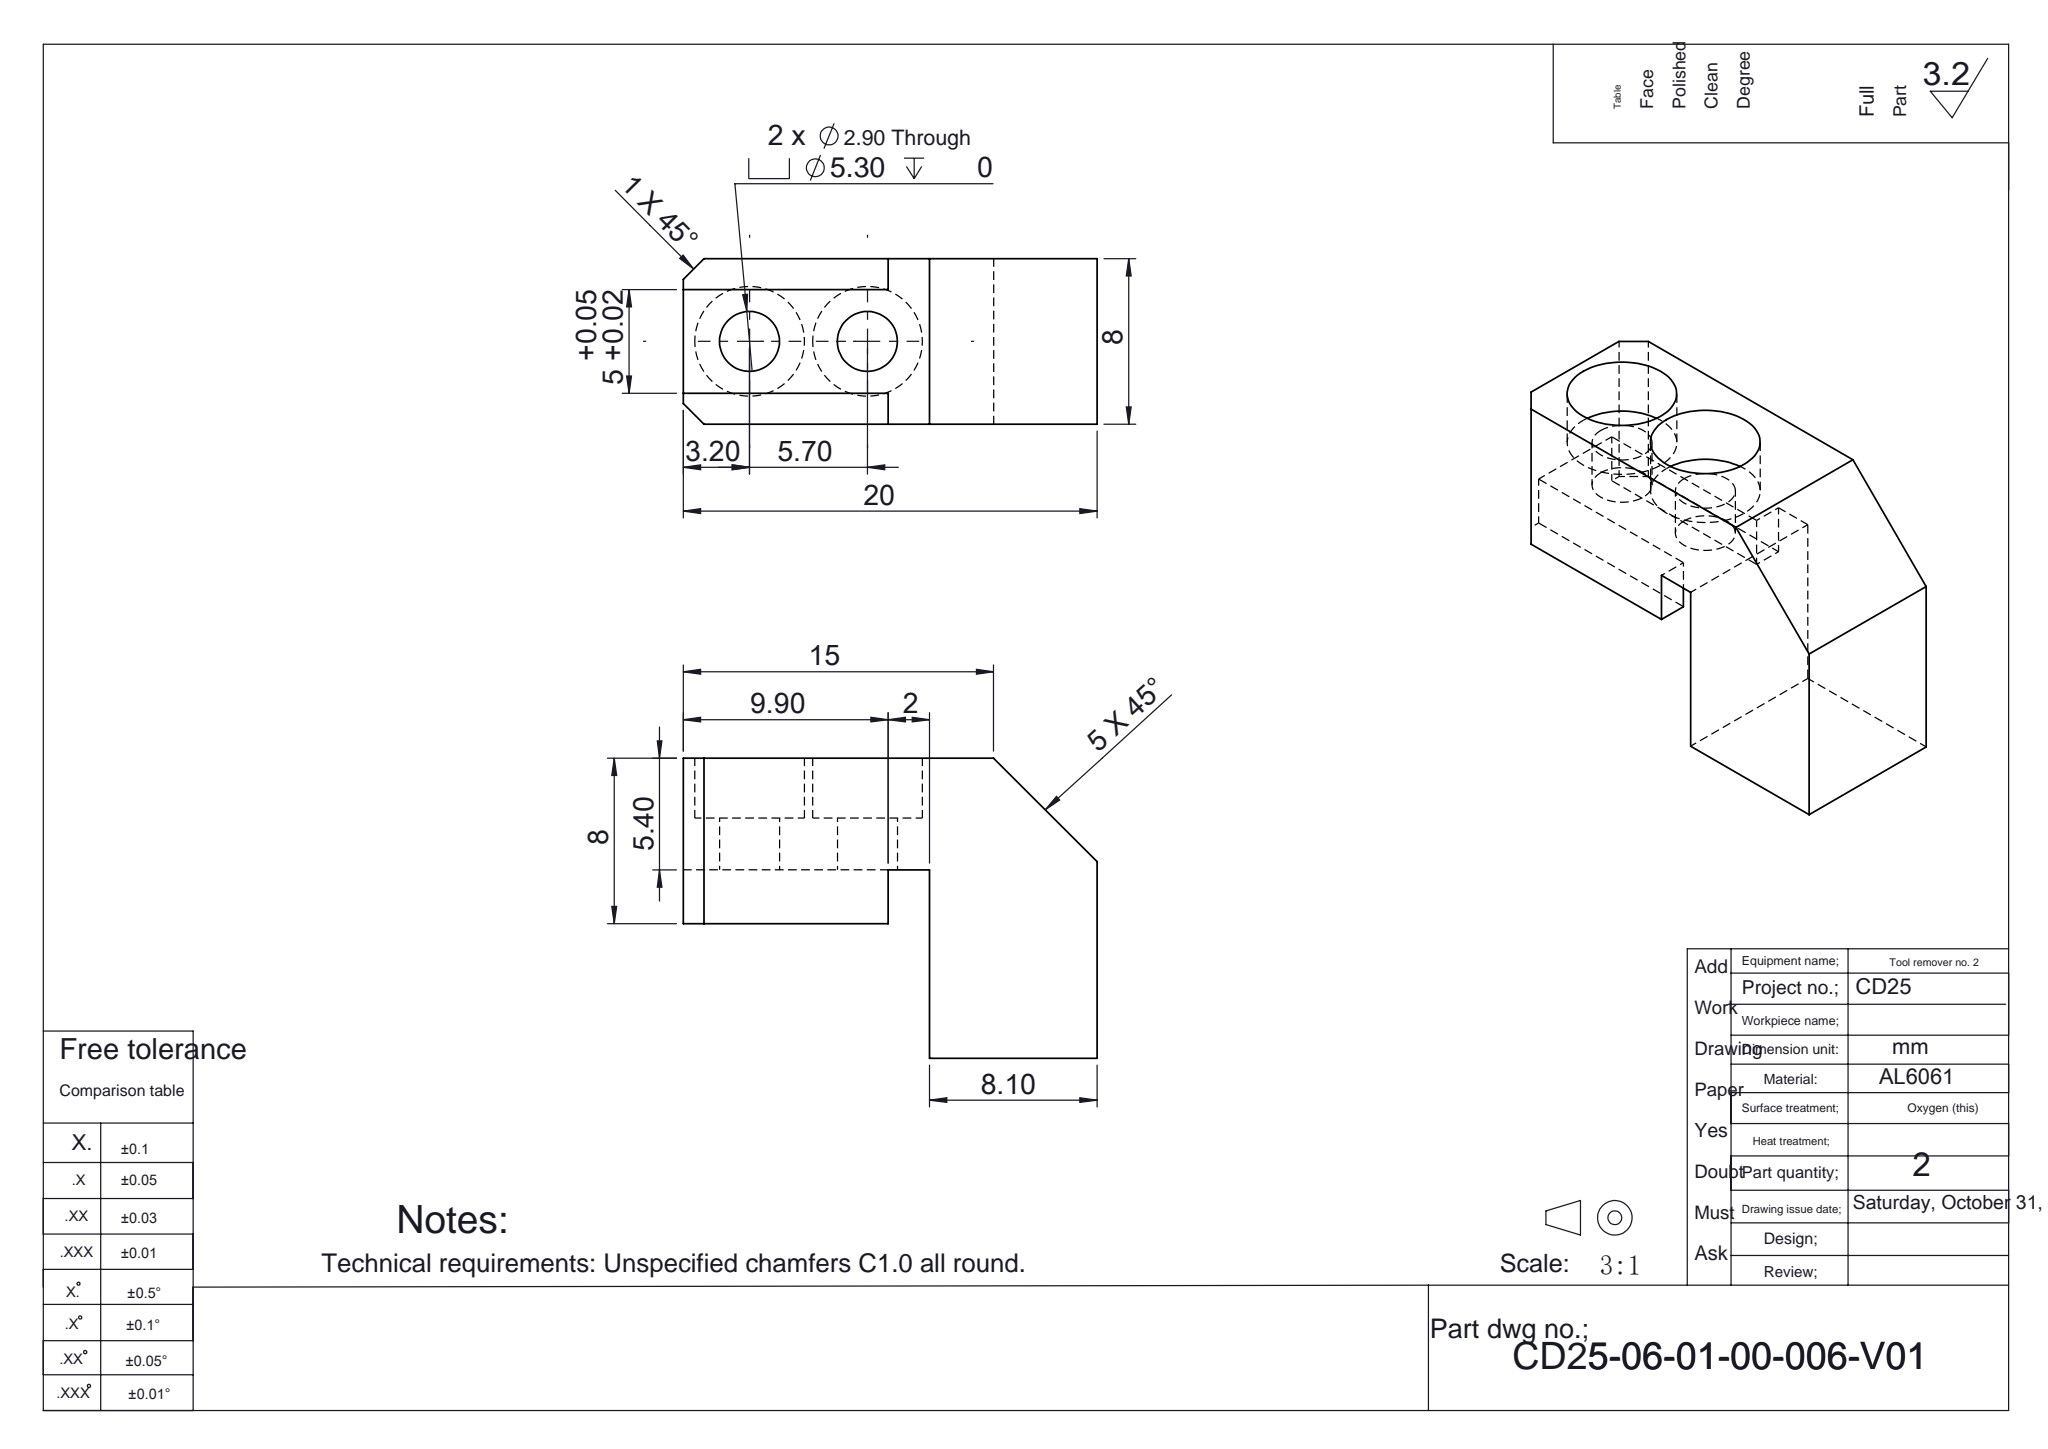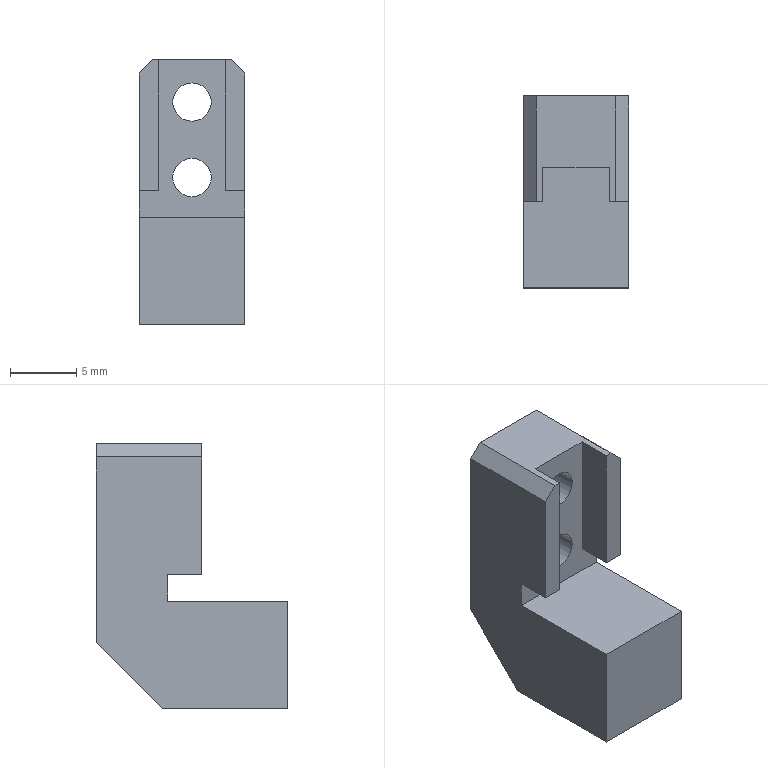Part | SolidWorks | features Chamfer 2, ICE 2, Cut 1, Extrusion 1, HoleWzd 1 | 1 solid | 27 faces | box 8 x 14.5 x 20 mm | volume 1262 mm3 | plane 19 | cylinder 8 | commonest cylinder face diameters 2.9 x4 5.3 x4
STEP:
#1=CARTESIAN_POINT('',(0.,4.35,4.15));
#2=VERTEX_POINT('',#1);
#3=CARTESIAN_POINT('',(0.,4.35,9.45));
#4=VERTEX_POINT('',#3);
#5=CARTESIAN_POINT('',(0.,4.35,6.8));
#6=DIRECTION('',(0.,1.,0.));
#7=DIRECTION('',(0.,0.,1.));
#8=AXIS2_PLACEMENT_3D('',#5,#6,#7);
#9=CIRCLE('',#8,2.65);
#10=EDGE_CURVE('',#2,#4,#9,.T.);
#11=ORIENTED_EDGE('',*,*,#10,.F.);
#12=CARTESIAN_POINT('',(0.,7.25,4.15));
#13=VERTEX_POINT('',#12);
#14=CARTESIAN_POINT('',(0.,7.25,4.15));
#15=DIRECTION('',(0.,1.,0.));
#16=VECTOR('',#15,1000.);
#17=LINE('',#14,#16);
#18=EDGE_CURVE('',#2,#13,#17,.T.);
#19=ORIENTED_EDGE('',*,*,#18,.T.);
#20=CARTESIAN_POINT('',(0.,7.25,9.45));
#21=VERTEX_POINT('',#20);
#22=CARTESIAN_POINT('',(0.,7.25,6.8));
#23=DIRECTION('',(0.,1.,0.));
#24=DIRECTION('',(0.,0.,1.));
#25=AXIS2_PLACEMENT_3D('',#22,#23,#24);
#26=CIRCLE('',#25,2.65);
#27=EDGE_CURVE('',#13,#21,#26,.T.);
#28=ORIENTED_EDGE('',*,*,#27,.T.);
#29=CARTESIAN_POINT('',(0.,7.25,9.45));
#30=DIRECTION('',(0.,1.,0.));
#31=VECTOR('',#30,1000.);
#32=LINE('',#29,#31);
#33=EDGE_CURVE('',#4,#21,#32,.T.);
#34=ORIENTED_EDGE('',*,*,#33,.F.);
#35=EDGE_LOOP('',(#11,#19,#28,#34));
#36=FACE_OUTER_BOUND('',#35,.T.);
#37=CARTESIAN_POINT('',(0.,7.25,6.8));
#38=DIRECTION('',(0.,1.,0.));
#39=DIRECTION('',(0.,0.,1.));
#40=AXIS2_PLACEMENT_3D('',#37,#38,#39);
#41=CYLINDRICAL_SURFACE('',#40,2.65);
#42=ADVANCED_FACE('',(#36),#41,.F.);
#43=CARTESIAN_POINT('',(0.,1.85,5.35));
#44=VERTEX_POINT('',#43);
#45=CARTESIAN_POINT('',(0.,1.85,8.25));
#46=VERTEX_POINT('',#45);
#47=CARTESIAN_POINT('',(0.,1.85,6.8));
#48=DIRECTION('',(0.,1.,0.));
#49=DIRECTION('',(0.,0.,1.));
#50=AXIS2_PLACEMENT_3D('',#47,#48,#49);
#51=CIRCLE('',#50,1.45);
#52=EDGE_CURVE('',#44,#46,#51,.T.);
#53=ORIENTED_EDGE('',*,*,#52,.F.);
#54=CARTESIAN_POINT('',(0.,4.35,5.35));
#55=VERTEX_POINT('',#54);
#56=CARTESIAN_POINT('',(0.,7.25,5.35));
#57=DIRECTION('',(0.,1.,0.));
#58=VECTOR('',#57,1000.);
#59=LINE('',#56,#58);
#60=EDGE_CURVE('',#44,#55,#59,.T.);
#61=ORIENTED_EDGE('',*,*,#60,.T.);
#62=CARTESIAN_POINT('',(0.,4.35,8.25));
#63=VERTEX_POINT('',#62);
#64=CARTESIAN_POINT('',(0.,4.35,6.8));
#65=DIRECTION('',(0.,1.,0.));
#66=DIRECTION('',(0.,0.,1.));
#67=AXIS2_PLACEMENT_3D('',#64,#65,#66);
#68=CIRCLE('',#67,1.45);
#69=EDGE_CURVE('',#55,#63,#68,.T.);
#70=ORIENTED_EDGE('',*,*,#69,.T.);
#71=CARTESIAN_POINT('',(0.,7.25,8.25));
#72=DIRECTION('',(0.,1.,0.));
#73=VECTOR('',#72,1000.);
#74=LINE('',#71,#73);
#75=EDGE_CURVE('',#46,#63,#74,.T.);
#76=ORIENTED_EDGE('',*,*,#75,.F.);
#77=EDGE_LOOP('',(#53,#61,#70,#76));
#78=FACE_OUTER_BOUND('',#77,.T.);
#79=CARTESIAN_POINT('',(0.,7.25,6.8));
#80=DIRECTION('',(0.,1.,0.));
#81=DIRECTION('',(0.,0.,1.));
#82=AXIS2_PLACEMENT_3D('',#79,#80,#81);
#83=CYLINDRICAL_SURFACE('',#82,1.45);
#84=ADVANCED_FACE('',(#78),#83,.F.);
#85=CARTESIAN_POINT('',(0.,4.35,-1.55));
#86=VERTEX_POINT('',#85);
#87=CARTESIAN_POINT('',(0.,4.35,3.75));
#88=VERTEX_POINT('',#87);
#89=CARTESIAN_POINT('',(0.,4.35,1.1));
#90=DIRECTION('',(0.,1.,0.));
#91=DIRECTION('',(0.,0.,1.));
#92=AXIS2_PLACEMENT_3D('',#89,#90,#91);
#93=CIRCLE('',#92,2.65);
#94=EDGE_CURVE('',#86,#88,#93,.T.);
#95=ORIENTED_EDGE('',*,*,#94,.F.);
#96=CARTESIAN_POINT('',(0.,7.25,-1.55));
#97=VERTEX_POINT('',#96);
#98=CARTESIAN_POINT('',(0.,7.25,-1.55));
#99=DIRECTION('',(0.,1.,0.));
#100=VECTOR('',#99,1000.);
#101=LINE('',#98,#100);
#102=EDGE_CURVE('',#86,#97,#101,.T.);
#103=ORIENTED_EDGE('',*,*,#102,.T.);
#104=CARTESIAN_POINT('',(0.,7.25,3.75));
#105=VERTEX_POINT('',#104);
#106=CARTESIAN_POINT('',(0.,7.25,1.1));
#107=DIRECTION('',(0.,1.,0.));
#108=DIRECTION('',(0.,0.,1.));
#109=AXIS2_PLACEMENT_3D('',#106,#107,#108);
#110=CIRCLE('',#109,2.65);
#111=EDGE_CURVE('',#97,#105,#110,.T.);
#112=ORIENTED_EDGE('',*,*,#111,.T.);
#113=CARTESIAN_POINT('',(0.,7.25,3.75));
#114=DIRECTION('',(0.,1.,0.));
#115=VECTOR('',#114,1000.);
#116=LINE('',#113,#115);
#117=EDGE_CURVE('',#88,#105,#116,.T.);
#118=ORIENTED_EDGE('',*,*,#117,.F.);
#119=EDGE_LOOP('',(#95,#103,#112,#118));
#120=FACE_OUTER_BOUND('',#119,.T.);
#121=CARTESIAN_POINT('',(0.,7.25,1.1));
#122=DIRECTION('',(0.,1.,0.));
#123=DIRECTION('',(0.,0.,1.));
#124=AXIS2_PLACEMENT_3D('',#121,#122,#123);
#125=CYLINDRICAL_SURFACE('',#124,2.65);
#126=ADVANCED_FACE('',(#120),#125,.F.);
#127=CARTESIAN_POINT('',(0.,1.85,-0.35));
#128=VERTEX_POINT('',#127);
#129=CARTESIAN_POINT('',(0.,1.85,2.55));
#130=VERTEX_POINT('',#129);
#131=CARTESIAN_POINT('',(0.,1.85,1.1));
#132=DIRECTION('',(0.,1.,0.));
#133=DIRECTION('',(0.,0.,1.));
#134=AXIS2_PLACEMENT_3D('',#131,#132,#133);
#135=CIRCLE('',#134,1.45);
#136=EDGE_CURVE('',#128,#130,#135,.T.);
#137=ORIENTED_EDGE('',*,*,#136,.F.);
#138=CARTESIAN_POINT('',(0.,4.35,-0.35));
#139=VERTEX_POINT('',#138);
#140=CARTESIAN_POINT('',(0.,7.25,-0.35));
#141=DIRECTION('',(0.,1.,0.));
#142=VECTOR('',#141,1000.);
#143=LINE('',#140,#142);
#144=EDGE_CURVE('',#128,#139,#143,.T.);
#145=ORIENTED_EDGE('',*,*,#144,.T.);
#146=CARTESIAN_POINT('',(0.,4.35,2.55));
#147=VERTEX_POINT('',#146);
#148=CARTESIAN_POINT('',(0.,4.35,1.1));
#149=DIRECTION('',(0.,1.,0.));
#150=DIRECTION('',(0.,0.,1.));
#151=AXIS2_PLACEMENT_3D('',#148,#149,#150);
#152=CIRCLE('',#151,1.45);
#153=EDGE_CURVE('',#139,#147,#152,.T.);
#154=ORIENTED_EDGE('',*,*,#153,.T.);
#155=CARTESIAN_POINT('',(0.,7.25,2.55));
#156=DIRECTION('',(0.,1.,0.));
#157=VECTOR('',#156,1000.);
#158=LINE('',#155,#157);
#159=EDGE_CURVE('',#130,#147,#158,.T.);
#160=ORIENTED_EDGE('',*,*,#159,.F.);
#161=EDGE_LOOP('',(#137,#145,#154,#160));
#162=FACE_OUTER_BOUND('',#161,.T.);
#163=CARTESIAN_POINT('',(0.,7.25,1.1));
#164=DIRECTION('',(0.,1.,0.));
#165=DIRECTION('',(0.,0.,1.));
#166=AXIS2_PLACEMENT_3D('',#163,#164,#165);
#167=CYLINDRICAL_SURFACE('',#166,1.45);
#168=ADVANCED_FACE('',(#162),#167,.F.);
#169=CARTESIAN_POINT('',(4.,1.85,0.1));
#170=VERTEX_POINT('',#169);
#171=CARTESIAN_POINT('',(4.,1.85,-1.9));
#172=VERTEX_POINT('',#171);
#173=CARTESIAN_POINT('',(4.,1.85,-10.));
#174=DIRECTION('',(0.,0.,-1.));
#175=VECTOR('',#174,1000.);
#176=LINE('',#173,#175);
#177=EDGE_CURVE('',#170,#172,#176,.T.);
#178=ORIENTED_EDGE('',*,*,#177,.T.);
#179=CARTESIAN_POINT('',(4.,-7.25,-1.9));
#180=VERTEX_POINT('',#179);
#181=CARTESIAN_POINT('',(4.,12.048,-1.9));
#182=DIRECTION('',(0.,-1.,0.));
#183=VECTOR('',#182,1000.);
#184=LINE('',#181,#183);
#185=EDGE_CURVE('',#172,#180,#184,.T.);
#186=ORIENTED_EDGE('',*,*,#185,.T.);
#187=CARTESIAN_POINT('',(4.,-7.25,-10.));
#188=VERTEX_POINT('',#187);
#189=CARTESIAN_POINT('',(4.,-7.25,-10.));
#190=DIRECTION('',(0.,0.,-1.));
#191=VECTOR('',#190,1000.);
#192=LINE('',#189,#191);
#193=EDGE_CURVE('',#180,#188,#192,.T.);
#194=ORIENTED_EDGE('',*,*,#193,.T.);
#195=CARTESIAN_POINT('',(4.,2.25,-10.));
#196=VERTEX_POINT('',#195);
#197=CARTESIAN_POINT('',(4.,7.25,-10.));
#198=DIRECTION('',(0.,-1.,0.));
#199=VECTOR('',#198,1000.);
#200=LINE('',#197,#199);
#201=EDGE_CURVE('',#196,#188,#200,.T.);
#202=ORIENTED_EDGE('',*,*,#201,.F.);
#203=CARTESIAN_POINT('',(4.,7.25,-5.));
#204=VERTEX_POINT('',#203);
#205=CARTESIAN_POINT('',(4.,7.25,-5.));
#206=DIRECTION('',(0.,0.7071,0.7071));
#207=VECTOR('',#206,1000.);
#208=LINE('',#205,#207);
#209=EDGE_CURVE('',#196,#204,#208,.T.);
#210=ORIENTED_EDGE('',*,*,#209,.T.);
#211=CARTESIAN_POINT('',(4.,7.25,9.));
#212=VERTEX_POINT('',#211);
#213=CARTESIAN_POINT('',(4.,7.25,-10.));
#214=DIRECTION('',(0.,0.,-1.));
#215=VECTOR('',#214,1000.);
#216=LINE('',#213,#215);
#217=EDGE_CURVE('',#212,#204,#216,.T.);
#218=ORIENTED_EDGE('',*,*,#217,.F.);
#219=CARTESIAN_POINT('',(4.,-0.75,9.));
#220=VERTEX_POINT('',#219);
#221=CARTESIAN_POINT('',(4.,7.25,9.));
#222=DIRECTION('',(0.,-1.,0.));
#223=VECTOR('',#222,1000.);
#224=LINE('',#221,#223);
#225=EDGE_CURVE('',#212,#220,#224,.T.);
#226=ORIENTED_EDGE('',*,*,#225,.T.);
#227=CARTESIAN_POINT('',(4.,-0.75,0.1));
#228=VERTEX_POINT('',#227);
#229=CARTESIAN_POINT('',(4.,-0.75,10.));
#230=DIRECTION('',(0.,0.,1.));
#231=VECTOR('',#230,1000.);
#232=LINE('',#229,#231);
#233=EDGE_CURVE('',#228,#220,#232,.T.);
#234=ORIENTED_EDGE('',*,*,#233,.F.);
#235=CARTESIAN_POINT('',(4.,12.048,0.1));
#236=DIRECTION('',(0.,-1.,0.));
#237=VECTOR('',#236,1000.);
#238=LINE('',#235,#237);
#239=EDGE_CURVE('',#170,#228,#238,.T.);
#240=ORIENTED_EDGE('',*,*,#239,.F.);
#241=EDGE_LOOP('',(#178,#186,#194,#202,#210,#218,#226,#234,#240));
#242=FACE_OUTER_BOUND('',#241,.T.);
#243=CARTESIAN_POINT('',(4.,7.25,-10.));
#244=DIRECTION('',(-1.,0.,0.));
#245=DIRECTION('',(0.,0.,1.));
#246=AXIS2_PLACEMENT_3D('',#243,#244,#245);
#247=PLANE('',#246);
#248=ADVANCED_FACE('',(#242),#247,.F.);
#249=CARTESIAN_POINT('',(-4.,2.25,-10.));
#250=VERTEX_POINT('',#249);
#251=CARTESIAN_POINT('',(-4.,-7.25,-10.));
#252=VERTEX_POINT('',#251);
#253=CARTESIAN_POINT('',(-4.,7.25,-10.));
#254=DIRECTION('',(0.,-1.,0.));
#255=VECTOR('',#254,1000.);
#256=LINE('',#253,#255);
#257=EDGE_CURVE('',#250,#252,#256,.T.);
#258=ORIENTED_EDGE('',*,*,#257,.F.);
#259=CARTESIAN_POINT('',(4.,2.25,-10.));
#260=DIRECTION('',(1.,0.,0.));
#261=VECTOR('',#260,1000.);
#262=LINE('',#259,#261);
#263=EDGE_CURVE('',#250,#196,#262,.T.);
#264=ORIENTED_EDGE('',*,*,#263,.T.);
#265=ORIENTED_EDGE('',*,*,#201,.T.);
#266=CARTESIAN_POINT('',(-4.,-7.25,-10.));
#267=DIRECTION('',(-1.,0.,0.));
#268=VECTOR('',#267,1000.);
#269=LINE('',#266,#268);
#270=EDGE_CURVE('',#188,#252,#269,.T.);
#271=ORIENTED_EDGE('',*,*,#270,.T.);
#272=EDGE_LOOP('',(#258,#264,#265,#271));
#273=FACE_OUTER_BOUND('',#272,.T.);
#274=CARTESIAN_POINT('',(-4.,7.25,-10.));
#275=DIRECTION('',(0.,0.,1.));
#276=DIRECTION('',(1.,0.,0.));
#277=AXIS2_PLACEMENT_3D('',#274,#275,#276);
#278=PLANE('',#277);
#279=ADVANCED_FACE('',(#273),#278,.F.);
#280=CARTESIAN_POINT('',(-4.,1.85,-1.9));
#281=VERTEX_POINT('',#280);
#282=CARTESIAN_POINT('',(-4.,1.85,0.1));
#283=VERTEX_POINT('',#282);
#284=CARTESIAN_POINT('',(-4.,1.85,-10.));
#285=DIRECTION('',(0.,0.,1.));
#286=VECTOR('',#285,1000.);
#287=LINE('',#284,#286);
#288=EDGE_CURVE('',#281,#283,#287,.T.);
#289=ORIENTED_EDGE('',*,*,#288,.T.);
#290=CARTESIAN_POINT('',(-4.,-0.75,0.1));
#291=VERTEX_POINT('',#290);
#292=CARTESIAN_POINT('',(-4.,12.048,0.1));
#293=DIRECTION('',(0.,-1.,0.));
#294=VECTOR('',#293,1000.);
#295=LINE('',#292,#294);
#296=EDGE_CURVE('',#283,#291,#295,.T.);
#297=ORIENTED_EDGE('',*,*,#296,.T.);
#298=CARTESIAN_POINT('',(-4.,-0.75,9.));
#299=VERTEX_POINT('',#298);
#300=CARTESIAN_POINT('',(-4.,-0.75,10.));
#301=DIRECTION('',(0.,0.,1.));
#302=VECTOR('',#301,1000.);
#303=LINE('',#300,#302);
#304=EDGE_CURVE('',#291,#299,#303,.T.);
#305=ORIENTED_EDGE('',*,*,#304,.T.);
#306=CARTESIAN_POINT('',(-4.,7.25,9.));
#307=VERTEX_POINT('',#306);
#308=CARTESIAN_POINT('',(-4.,7.25,9.));
#309=DIRECTION('',(0.,1.,0.));
#310=VECTOR('',#309,1000.);
#311=LINE('',#308,#310);
#312=EDGE_CURVE('',#299,#307,#311,.T.);
#313=ORIENTED_EDGE('',*,*,#312,.T.);
#314=CARTESIAN_POINT('',(-4.,7.25,-5.));
#315=VERTEX_POINT('',#314);
#316=CARTESIAN_POINT('',(-4.,7.25,-10.));
#317=DIRECTION('',(0.,0.,1.));
#318=VECTOR('',#317,1000.);
#319=LINE('',#316,#318);
#320=EDGE_CURVE('',#315,#307,#319,.T.);
#321=ORIENTED_EDGE('',*,*,#320,.F.);
#322=CARTESIAN_POINT('',(-4.,7.25,-5.));
#323=DIRECTION('',(0.,-0.7071,-0.7071));
#324=VECTOR('',#323,1000.);
#325=LINE('',#322,#324);
#326=EDGE_CURVE('',#315,#250,#325,.T.);
#327=ORIENTED_EDGE('',*,*,#326,.T.);
#328=ORIENTED_EDGE('',*,*,#257,.T.);
#329=CARTESIAN_POINT('',(-4.,-7.25,-1.9));
#330=VERTEX_POINT('',#329);
#331=CARTESIAN_POINT('',(-4.,-7.25,-10.));
#332=DIRECTION('',(0.,0.,1.));
#333=VECTOR('',#332,1000.);
#334=LINE('',#331,#333);
#335=EDGE_CURVE('',#252,#330,#334,.T.);
#336=ORIENTED_EDGE('',*,*,#335,.T.);
#337=CARTESIAN_POINT('',(-4.,12.048,-1.9));
#338=DIRECTION('',(0.,-1.,0.));
#339=VECTOR('',#338,1000.);
#340=LINE('',#337,#339);
#341=EDGE_CURVE('',#281,#330,#340,.T.);
#342=ORIENTED_EDGE('',*,*,#341,.F.);
#343=EDGE_LOOP('',(#289,#297,#305,#313,#321,#327,#328,#336,#342));
#344=FACE_OUTER_BOUND('',#343,.T.);
#345=CARTESIAN_POINT('',(-4.,7.25,-10.));
#346=DIRECTION('',(1.,0.,0.));
#347=DIRECTION('',(0.,0.,-1.));
#348=AXIS2_PLACEMENT_3D('',#345,#346,#347);
#349=PLANE('',#348);
#350=ADVANCED_FACE('',(#344),#349,.F.);
#351=CARTESIAN_POINT('',(-3.,7.25,10.));
#352=VERTEX_POINT('',#351);
#353=CARTESIAN_POINT('',(3.,7.25,10.));
#354=VERTEX_POINT('',#353);
#355=CARTESIAN_POINT('',(-4.,7.25,10.));
#356=DIRECTION('',(1.,0.,0.));
#357=VECTOR('',#356,1000.);
#358=LINE('',#355,#357);
#359=EDGE_CURVE('',#352,#354,#358,.T.);
#360=ORIENTED_EDGE('',*,*,#359,.F.);
#361=CARTESIAN_POINT('',(-3.,-0.75,10.));
#362=VERTEX_POINT('',#361);
#363=CARTESIAN_POINT('',(-3.,7.25,10.));
#364=DIRECTION('',(0.,-1.,0.));
#365=VECTOR('',#364,1000.);
#366=LINE('',#363,#365);
#367=EDGE_CURVE('',#352,#362,#366,.T.);
#368=ORIENTED_EDGE('',*,*,#367,.T.);
#369=CARTESIAN_POINT('',(-2.5,-0.75,10.));
#370=VERTEX_POINT('',#369);
#371=CARTESIAN_POINT('',(-4.,-0.75,10.));
#372=DIRECTION('',(1.,0.,0.));
#373=VECTOR('',#372,1000.);
#374=LINE('',#371,#373);
#375=EDGE_CURVE('',#362,#370,#374,.T.);
#376=ORIENTED_EDGE('',*,*,#375,.T.);
#377=CARTESIAN_POINT('',(-2.5,1.85,10.));
#378=VERTEX_POINT('',#377);
#379=CARTESIAN_POINT('',(-2.5,20.158,10.));
#380=DIRECTION('',(0.,-1.,0.));
#381=VECTOR('',#380,1000.);
#382=LINE('',#379,#381);
#383=EDGE_CURVE('',#378,#370,#382,.T.);
#384=ORIENTED_EDGE('',*,*,#383,.F.);
#385=CARTESIAN_POINT('',(2.5,1.85,10.));
#386=VERTEX_POINT('',#385);
#387=CARTESIAN_POINT('',(-2.5,1.85,10.));
#388=DIRECTION('',(-1.,0.,0.));
#389=VECTOR('',#388,1000.);
#390=LINE('',#387,#389);
#391=EDGE_CURVE('',#386,#378,#390,.T.);
#392=ORIENTED_EDGE('',*,*,#391,.F.);
#393=CARTESIAN_POINT('',(2.5,-0.75,10.));
#394=VERTEX_POINT('',#393);
#395=CARTESIAN_POINT('',(2.5,20.158,10.));
#396=DIRECTION('',(0.,-1.,0.));
#397=VECTOR('',#396,1000.);
#398=LINE('',#395,#397);
#399=EDGE_CURVE('',#386,#394,#398,.T.);
#400=ORIENTED_EDGE('',*,*,#399,.T.);
#401=CARTESIAN_POINT('',(3.,-0.75,10.));
#402=VERTEX_POINT('',#401);
#403=CARTESIAN_POINT('',(-4.,-0.75,10.));
#404=DIRECTION('',(1.,0.,0.));
#405=VECTOR('',#404,1000.);
#406=LINE('',#403,#405);
#407=EDGE_CURVE('',#394,#402,#406,.T.);
#408=ORIENTED_EDGE('',*,*,#407,.T.);
#409=CARTESIAN_POINT('',(3.,7.25,10.));
#410=DIRECTION('',(0.,1.,0.));
#411=VECTOR('',#410,1000.);
#412=LINE('',#409,#411);
#413=EDGE_CURVE('',#402,#354,#412,.T.);
#414=ORIENTED_EDGE('',*,*,#413,.T.);
#415=EDGE_LOOP('',(#360,#368,#376,#384,#392,#400,#408,#414));
#416=FACE_OUTER_BOUND('',#415,.T.);
#417=CARTESIAN_POINT('',(-4.,7.25,10.));
#418=DIRECTION('',(0.,0.,-1.));
#419=DIRECTION('',(-1.,0.,0.));
#420=AXIS2_PLACEMENT_3D('',#417,#418,#419);
#421=PLANE('',#420);
#422=ADVANCED_FACE('',(#416),#421,.F.);
#423=CARTESIAN_POINT('',(0.,7.25,6.8));
#424=DIRECTION('',(0.,1.,0.));
#425=DIRECTION('',(0.,0.,1.));
#426=AXIS2_PLACEMENT_3D('',#423,#424,#425);
#427=CIRCLE('',#426,2.65);
#428=EDGE_CURVE('',#21,#13,#427,.T.);
#429=ORIENTED_EDGE('',*,*,#428,.F.);
#430=ORIENTED_EDGE('',*,*,#27,.F.);
#431=EDGE_LOOP('',(#429,#430));
#432=FACE_BOUND('',#431,.T.);
#433=CARTESIAN_POINT('',(0.,7.25,1.1));
#434=DIRECTION('',(0.,1.,0.));
#435=DIRECTION('',(0.,0.,1.));
#436=AXIS2_PLACEMENT_3D('',#433,#434,#435);
#437=CIRCLE('',#436,2.65);
#438=EDGE_CURVE('',#105,#97,#437,.T.);
#439=ORIENTED_EDGE('',*,*,#438,.F.);
#440=ORIENTED_EDGE('',*,*,#111,.F.);
#441=EDGE_LOOP('',(#439,#440));
#442=FACE_BOUND('',#441,.T.);
#443=ORIENTED_EDGE('',*,*,#217,.T.);
#444=CARTESIAN_POINT('',(-4.,7.25,-5.));
#445=DIRECTION('',(-1.,0.,0.));
#446=VECTOR('',#445,1000.);
#447=LINE('',#444,#446);
#448=EDGE_CURVE('',#204,#315,#447,.T.);
#449=ORIENTED_EDGE('',*,*,#448,.T.);
#450=ORIENTED_EDGE('',*,*,#320,.T.);
#451=CARTESIAN_POINT('',(-6.5,7.25,6.5));
#452=DIRECTION('',(0.7071,0.,0.7071));
#453=VECTOR('',#452,1000.);
#454=LINE('',#451,#453);
#455=EDGE_CURVE('',#307,#352,#454,.T.);
#456=ORIENTED_EDGE('',*,*,#455,.T.);
#457=ORIENTED_EDGE('',*,*,#359,.T.);
#458=CARTESIAN_POINT('',(6.5,7.25,6.5));
#459=DIRECTION('',(0.7071,0.,-0.7071));
#460=VECTOR('',#459,1000.);
#461=LINE('',#458,#460);
#462=EDGE_CURVE('',#354,#212,#461,.T.);
#463=ORIENTED_EDGE('',*,*,#462,.T.);
#464=EDGE_LOOP('',(#443,#449,#450,#456,#457,#463));
#465=FACE_OUTER_BOUND('',#464,.T.);
#466=CARTESIAN_POINT('',(0.,7.25,0.));
#467=DIRECTION('',(0.,1.,0.));
#468=DIRECTION('',(0.,0.,1.));
#469=AXIS2_PLACEMENT_3D('',#466,#467,#468);
#470=PLANE('',#469);
#471=ADVANCED_FACE('',(#432,#442,#465),#470,.T.);
#472=ORIENTED_EDGE('',*,*,#193,.F.);
#473=CARTESIAN_POINT('',(-2.5,-7.25,-1.9));
#474=DIRECTION('',(1.,0.,0.));
#475=VECTOR('',#474,1000.);
#476=LINE('',#473,#475);
#477=EDGE_CURVE('',#330,#180,#476,.T.);
#478=ORIENTED_EDGE('',*,*,#477,.F.);
#479=ORIENTED_EDGE('',*,*,#335,.F.);
#480=ORIENTED_EDGE('',*,*,#270,.F.);
#481=EDGE_LOOP('',(#472,#478,#479,#480));
#482=FACE_OUTER_BOUND('',#481,.T.);
#483=CARTESIAN_POINT('',(0.,-7.25,0.));
#484=DIRECTION('',(0.,1.,0.));
#485=DIRECTION('',(0.,0.,1.));
#486=AXIS2_PLACEMENT_3D('',#483,#484,#485);
#487=PLANE('',#486);
#488=ADVANCED_FACE('',(#482),#487,.F.);
#489=CARTESIAN_POINT('',(0.,1.85,1.1));
#490=DIRECTION('',(0.,1.,0.));
#491=DIRECTION('',(0.,0.,1.));
#492=AXIS2_PLACEMENT_3D('',#489,#490,#491);
#493=CIRCLE('',#492,1.45);
#494=EDGE_CURVE('',#130,#128,#493,.T.);
#495=ORIENTED_EDGE('',*,*,#494,.T.);
#496=ORIENTED_EDGE('',*,*,#136,.T.);
#497=EDGE_LOOP('',(#495,#496));
#498=FACE_BOUND('',#497,.T.);
#499=CARTESIAN_POINT('',(0.,1.85,6.8));
#500=DIRECTION('',(0.,1.,0.));
#501=DIRECTION('',(0.,0.,1.));
#502=AXIS2_PLACEMENT_3D('',#499,#500,#501);
#503=CIRCLE('',#502,1.45);
#504=EDGE_CURVE('',#46,#44,#503,.T.);
#505=ORIENTED_EDGE('',*,*,#504,.T.);
#506=ORIENTED_EDGE('',*,*,#52,.T.);
#507=EDGE_LOOP('',(#505,#506));
#508=FACE_BOUND('',#507,.T.);
#509=CARTESIAN_POINT('',(-2.5,1.85,0.1));
#510=VERTEX_POINT('',#509);
#511=CARTESIAN_POINT('',(-2.5,1.85,10.));
#512=DIRECTION('',(0.,0.,-1.));
#513=VECTOR('',#512,1000.);
#514=LINE('',#511,#513);
#515=EDGE_CURVE('',#378,#510,#514,.T.);
#516=ORIENTED_EDGE('',*,*,#515,.T.);
#517=CARTESIAN_POINT('',(-4.,1.85,0.1));
#518=DIRECTION('',(-1.,0.,0.));
#519=VECTOR('',#518,1000.);
#520=LINE('',#517,#519);
#521=EDGE_CURVE('',#510,#283,#520,.T.);
#522=ORIENTED_EDGE('',*,*,#521,.T.);
#523=ORIENTED_EDGE('',*,*,#288,.F.);
#524=CARTESIAN_POINT('',(-2.5,1.85,-1.9));
#525=DIRECTION('',(1.,0.,0.));
#526=VECTOR('',#525,1000.);
#527=LINE('',#524,#526);
#528=EDGE_CURVE('',#281,#172,#527,.T.);
#529=ORIENTED_EDGE('',*,*,#528,.T.);
#530=ORIENTED_EDGE('',*,*,#177,.F.);
#531=CARTESIAN_POINT('',(2.5,1.85,0.1));
#532=VERTEX_POINT('',#531);
#533=CARTESIAN_POINT('',(-4.,1.85,0.1));
#534=DIRECTION('',(-1.,0.,0.));
#535=VECTOR('',#534,1000.);
#536=LINE('',#533,#535);
#537=EDGE_CURVE('',#170,#532,#536,.T.);
#538=ORIENTED_EDGE('',*,*,#537,.T.);
#539=CARTESIAN_POINT('',(2.5,1.85,10.));
#540=DIRECTION('',(0.,0.,1.));
#541=VECTOR('',#540,1000.);
#542=LINE('',#539,#541);
#543=EDGE_CURVE('',#532,#386,#542,.T.);
#544=ORIENTED_EDGE('',*,*,#543,.T.);
#545=ORIENTED_EDGE('',*,*,#391,.T.);
#546=EDGE_LOOP('',(#516,#522,#523,#529,#530,#538,#544,#545));
#547=FACE_OUTER_BOUND('',#546,.T.);
#548=CARTESIAN_POINT('',(0.,1.85,0.));
#549=DIRECTION('',(0.,1.,0.));
#550=DIRECTION('',(0.,0.,1.));
#551=AXIS2_PLACEMENT_3D('',#548,#549,#550);
#552=PLANE('',#551);
#553=ADVANCED_FACE('',(#498,#508,#547),#552,.F.);
#554=ORIENTED_EDGE('',*,*,#528,.F.);
#555=ORIENTED_EDGE('',*,*,#341,.T.);
#556=ORIENTED_EDGE('',*,*,#477,.T.);
#557=ORIENTED_EDGE('',*,*,#185,.F.);
#558=EDGE_LOOP('',(#554,#555,#556,#557));
#559=FACE_OUTER_BOUND('',#558,.T.);
#560=CARTESIAN_POINT('',(-2.5,20.158,-1.9));
#561=DIRECTION('',(0.,0.,-1.));
#562=DIRECTION('',(-1.,0.,0.));
#563=AXIS2_PLACEMENT_3D('',#560,#561,#562);
#564=PLANE('',#563);
#565=ADVANCED_FACE('',(#559),#564,.F.);
#566=ORIENTED_EDGE('',*,*,#543,.F.);
#567=CARTESIAN_POINT('',(2.5,-0.75,0.1));
#568=VERTEX_POINT('',#567);
#569=CARTESIAN_POINT('',(2.5,20.158,0.1));
#570=DIRECTION('',(0.,-1.,0.));
#571=VECTOR('',#570,1000.);
#572=LINE('',#569,#571);
#573=EDGE_CURVE('',#532,#568,#572,.T.);
#574=ORIENTED_EDGE('',*,*,#573,.T.);
#575=CARTESIAN_POINT('',(2.5,-0.75,10.));
#576=DIRECTION('',(0.,0.,1.));
#577=VECTOR('',#576,1000.);
#578=LINE('',#575,#577);
#579=EDGE_CURVE('',#568,#394,#578,.T.);
#580=ORIENTED_EDGE('',*,*,#579,.T.);
#581=ORIENTED_EDGE('',*,*,#399,.F.);
#582=EDGE_LOOP('',(#566,#574,#580,#581));
#583=FACE_OUTER_BOUND('',#582,.T.);
#584=CARTESIAN_POINT('',(2.5,20.158,10.));
#585=DIRECTION('',(1.,0.,0.));
#586=DIRECTION('',(0.,0.,-1.));
#587=AXIS2_PLACEMENT_3D('',#584,#585,#586);
#588=PLANE('',#587);
#589=ADVANCED_FACE('',(#583),#588,.F.);
#590=CARTESIAN_POINT('',(-2.5,-0.75,0.1));
#591=VERTEX_POINT('',#590);
#592=CARTESIAN_POINT('',(-2.5,-0.75,10.));
#593=DIRECTION('',(0.,0.,-1.));
#594=VECTOR('',#593,1000.);
#595=LINE('',#592,#594);
#596=EDGE_CURVE('',#370,#591,#595,.T.);
#597=ORIENTED_EDGE('',*,*,#596,.T.);
#598=CARTESIAN_POINT('',(-2.5,20.158,0.1));
#599=DIRECTION('',(0.,1.,0.));
#600=VECTOR('',#599,1000.);
#601=LINE('',#598,#600);
#602=EDGE_CURVE('',#591,#510,#601,.T.);
#603=ORIENTED_EDGE('',*,*,#602,.T.);
#604=ORIENTED_EDGE('',*,*,#515,.F.);
#605=ORIENTED_EDGE('',*,*,#383,.T.);
#606=EDGE_LOOP('',(#597,#603,#604,#605));
#607=FACE_OUTER_BOUND('',#606,.T.);
#608=CARTESIAN_POINT('',(-2.5,20.158,10.));
#609=DIRECTION('',(-1.,0.,0.));
#610=DIRECTION('',(0.,0.,1.));
#611=AXIS2_PLACEMENT_3D('',#608,#609,#610);
#612=PLANE('',#611);
#613=ADVANCED_FACE('',(#607),#612,.F.);
#614=ORIENTED_EDGE('',*,*,#144,.F.);
#615=ORIENTED_EDGE('',*,*,#494,.F.);
#616=ORIENTED_EDGE('',*,*,#159,.T.);
#617=CARTESIAN_POINT('',(0.,4.35,1.1));
#618=DIRECTION('',(0.,1.,0.));
#619=DIRECTION('',(0.,0.,1.));
#620=AXIS2_PLACEMENT_3D('',#617,#618,#619);
#621=CIRCLE('',#620,1.45);
#622=EDGE_CURVE('',#147,#139,#621,.T.);
#623=ORIENTED_EDGE('',*,*,#622,.T.);
#624=EDGE_LOOP('',(#614,#615,#616,#623));
#625=FACE_OUTER_BOUND('',#624,.T.);
#626=CARTESIAN_POINT('',(0.,7.25,1.1));
#627=DIRECTION('',(0.,1.,0.));
#628=DIRECTION('',(0.,0.,1.));
#629=AXIS2_PLACEMENT_3D('',#626,#627,#628);
#630=CYLINDRICAL_SURFACE('',#629,1.45);
#631=ADVANCED_FACE('',(#625),#630,.F.);
#632=ORIENTED_EDGE('',*,*,#622,.F.);
#633=ORIENTED_EDGE('',*,*,#153,.F.);
#634=EDGE_LOOP('',(#632,#633));
#635=FACE_BOUND('',#634,.T.);
#636=CARTESIAN_POINT('',(0.,4.35,1.1));
#637=DIRECTION('',(0.,1.,0.));
#638=DIRECTION('',(0.,0.,1.));
#639=AXIS2_PLACEMENT_3D('',#636,#637,#638);
#640=CIRCLE('',#639,2.65);
#641=EDGE_CURVE('',#88,#86,#640,.T.);
#642=ORIENTED_EDGE('',*,*,#641,.T.);
#643=ORIENTED_EDGE('',*,*,#94,.T.);
#644=EDGE_LOOP('',(#642,#643));
#645=FACE_OUTER_BOUND('',#644,.T.);
#646=CARTESIAN_POINT('',(1.45,4.35,1.1));
#647=DIRECTION('',(0.,-1.,0.));
#648=DIRECTION('',(0.,0.,-1.));
#649=AXIS2_PLACEMENT_3D('',#646,#647,#648);
#650=PLANE('',#649);
#651=ADVANCED_FACE('',(#635,#645),#650,.F.);
#652=ORIENTED_EDGE('',*,*,#102,.F.);
#653=ORIENTED_EDGE('',*,*,#641,.F.);
#654=ORIENTED_EDGE('',*,*,#117,.T.);
#655=ORIENTED_EDGE('',*,*,#438,.T.);
#656=EDGE_LOOP('',(#652,#653,#654,#655));
#657=FACE_OUTER_BOUND('',#656,.T.);
#658=CARTESIAN_POINT('',(0.,7.25,1.1));
#659=DIRECTION('',(0.,1.,0.));
#660=DIRECTION('',(0.,0.,1.));
#661=AXIS2_PLACEMENT_3D('',#658,#659,#660);
#662=CYLINDRICAL_SURFACE('',#661,2.65);
#663=ADVANCED_FACE('',(#657),#662,.F.);
#664=ORIENTED_EDGE('',*,*,#60,.F.);
#665=ORIENTED_EDGE('',*,*,#504,.F.);
#666=ORIENTED_EDGE('',*,*,#75,.T.);
#667=CARTESIAN_POINT('',(0.,4.35,6.8));
#668=DIRECTION('',(0.,1.,0.));
#669=DIRECTION('',(0.,0.,1.));
#670=AXIS2_PLACEMENT_3D('',#667,#668,#669);
#671=CIRCLE('',#670,1.45);
#672=EDGE_CURVE('',#63,#55,#671,.T.);
#673=ORIENTED_EDGE('',*,*,#672,.T.);
#674=EDGE_LOOP('',(#664,#665,#666,#673));
#675=FACE_OUTER_BOUND('',#674,.T.);
#676=CARTESIAN_POINT('',(0.,7.25,6.8));
#677=DIRECTION('',(0.,1.,0.));
#678=DIRECTION('',(0.,0.,1.));
#679=AXIS2_PLACEMENT_3D('',#676,#677,#678);
#680=CYLINDRICAL_SURFACE('',#679,1.45);
#681=ADVANCED_FACE('',(#675),#680,.F.);
#682=ORIENTED_EDGE('',*,*,#672,.F.);
#683=ORIENTED_EDGE('',*,*,#69,.F.);
#684=EDGE_LOOP('',(#682,#683));
#685=FACE_BOUND('',#684,.T.);
#686=CARTESIAN_POINT('',(0.,4.35,6.8));
#687=DIRECTION('',(0.,1.,0.));
#688=DIRECTION('',(0.,0.,1.));
#689=AXIS2_PLACEMENT_3D('',#686,#687,#688);
#690=CIRCLE('',#689,2.65);
#691=EDGE_CURVE('',#4,#2,#690,.T.);
#692=ORIENTED_EDGE('',*,*,#691,.T.);
#693=ORIENTED_EDGE('',*,*,#10,.T.);
#694=EDGE_LOOP('',(#692,#693));
#695=FACE_OUTER_BOUND('',#694,.T.);
#696=CARTESIAN_POINT('',(1.45,4.35,6.8));
#697=DIRECTION('',(0.,-1.,0.));
#698=DIRECTION('',(0.,0.,-1.));
#699=AXIS2_PLACEMENT_3D('',#696,#697,#698);
#700=PLANE('',#699);
#701=ADVANCED_FACE('',(#685,#695),#700,.F.);
#702=ORIENTED_EDGE('',*,*,#18,.F.);
#703=ORIENTED_EDGE('',*,*,#691,.F.);
#704=ORIENTED_EDGE('',*,*,#33,.T.);
#705=ORIENTED_EDGE('',*,*,#428,.T.);
#706=EDGE_LOOP('',(#702,#703,#704,#705));
#707=FACE_OUTER_BOUND('',#706,.T.);
#708=CARTESIAN_POINT('',(0.,7.25,6.8));
#709=DIRECTION('',(0.,1.,0.));
#710=DIRECTION('',(0.,0.,1.));
#711=AXIS2_PLACEMENT_3D('',#708,#709,#710);
#712=CYLINDRICAL_SURFACE('',#711,2.65);
#713=ADVANCED_FACE('',(#707),#712,.F.);
#714=ORIENTED_EDGE('',*,*,#304,.F.);
#715=CARTESIAN_POINT('',(-4.,-0.75,0.1));
#716=DIRECTION('',(1.,0.,0.));
#717=VECTOR('',#716,1000.);
#718=LINE('',#715,#717);
#719=EDGE_CURVE('',#291,#591,#718,.T.);
#720=ORIENTED_EDGE('',*,*,#719,.T.);
#721=ORIENTED_EDGE('',*,*,#596,.F.);
#722=ORIENTED_EDGE('',*,*,#375,.F.);
#723=CARTESIAN_POINT('',(-3.,-0.75,10.));
#724=DIRECTION('',(-0.7071,0.,-0.7071));
#725=VECTOR('',#724,1000.);
#726=LINE('',#723,#725);
#727=EDGE_CURVE('',#362,#299,#726,.T.);
#728=ORIENTED_EDGE('',*,*,#727,.T.);
#729=EDGE_LOOP('',(#714,#720,#721,#722,#728));
#730=FACE_OUTER_BOUND('',#729,.T.);
#731=CARTESIAN_POINT('',(-4.,-0.75,10.));
#732=DIRECTION('',(0.,1.,0.));
#733=DIRECTION('',(0.,0.,1.));
#734=AXIS2_PLACEMENT_3D('',#731,#732,#733);
#735=PLANE('',#734);
#736=ADVANCED_FACE('',(#730),#735,.F.);
#737=ORIENTED_EDGE('',*,*,#579,.F.);
#738=CARTESIAN_POINT('',(-4.,-0.75,0.1));
#739=DIRECTION('',(1.,0.,0.));
#740=VECTOR('',#739,1000.);
#741=LINE('',#738,#740);
#742=EDGE_CURVE('',#568,#228,#741,.T.);
#743=ORIENTED_EDGE('',*,*,#742,.T.);
#744=ORIENTED_EDGE('',*,*,#233,.T.);
#745=CARTESIAN_POINT('',(4.,-0.75,9.));
#746=DIRECTION('',(-0.7071,0.,0.7071));
#747=VECTOR('',#746,1000.);
#748=LINE('',#745,#747);
#749=EDGE_CURVE('',#220,#402,#748,.T.);
#750=ORIENTED_EDGE('',*,*,#749,.T.);
#751=ORIENTED_EDGE('',*,*,#407,.F.);
#752=EDGE_LOOP('',(#737,#743,#744,#750,#751));
#753=FACE_OUTER_BOUND('',#752,.T.);
#754=CARTESIAN_POINT('',(-4.,-0.75,10.));
#755=DIRECTION('',(0.,1.,0.));
#756=DIRECTION('',(0.,0.,1.));
#757=AXIS2_PLACEMENT_3D('',#754,#755,#756);
#758=PLANE('',#757);
#759=ADVANCED_FACE('',(#753),#758,.F.);
#760=ORIENTED_EDGE('',*,*,#455,.F.);
#761=ORIENTED_EDGE('',*,*,#312,.F.);
#762=ORIENTED_EDGE('',*,*,#727,.F.);
#763=ORIENTED_EDGE('',*,*,#367,.F.);
#764=EDGE_LOOP('',(#760,#761,#762,#763));
#765=FACE_OUTER_BOUND('',#764,.T.);
#766=CARTESIAN_POINT('',(-3.,7.25,10.));
#767=DIRECTION('',(0.7071,0.,-0.7071));
#768=DIRECTION('',(0.,-1.,0.));
#769=AXIS2_PLACEMENT_3D('',#766,#767,#768);
#770=PLANE('',#769);
#771=ADVANCED_FACE('',(#765),#770,.F.);
#772=ORIENTED_EDGE('',*,*,#462,.F.);
#773=ORIENTED_EDGE('',*,*,#413,.F.);
#774=ORIENTED_EDGE('',*,*,#749,.F.);
#775=ORIENTED_EDGE('',*,*,#225,.F.);
#776=EDGE_LOOP('',(#772,#773,#774,#775));
#777=FACE_OUTER_BOUND('',#776,.T.);
#778=CARTESIAN_POINT('',(4.,7.25,9.));
#779=DIRECTION('',(-0.7071,0.,-0.7071));
#780=DIRECTION('',(0.,-1.,0.));
#781=AXIS2_PLACEMENT_3D('',#778,#779,#780);
#782=PLANE('',#781);
#783=ADVANCED_FACE('',(#777),#782,.F.);
#784=ORIENTED_EDGE('',*,*,#209,.F.);
#785=ORIENTED_EDGE('',*,*,#263,.F.);
#786=ORIENTED_EDGE('',*,*,#326,.F.);
#787=ORIENTED_EDGE('',*,*,#448,.F.);
#788=EDGE_LOOP('',(#784,#785,#786,#787));
#789=FACE_OUTER_BOUND('',#788,.T.);
#790=CARTESIAN_POINT('',(0.,7.25,-5.));
#791=DIRECTION('',(0.,0.7071,-0.7071));
#792=DIRECTION('',(1.,0.,0.));
#793=AXIS2_PLACEMENT_3D('',#790,#791,#792);
#794=PLANE('',#793);
#795=ADVANCED_FACE('',(#789),#794,.T.);
#796=ORIENTED_EDGE('',*,*,#537,.F.);
#797=ORIENTED_EDGE('',*,*,#239,.T.);
#798=ORIENTED_EDGE('',*,*,#742,.F.);
#799=ORIENTED_EDGE('',*,*,#573,.F.);
#800=EDGE_LOOP('',(#796,#797,#798,#799));
#801=FACE_OUTER_BOUND('',#800,.T.);
#802=CARTESIAN_POINT('',(-4.,12.048,0.1));
#803=DIRECTION('',(0.,0.,1.));
#804=DIRECTION('',(1.,0.,0.));
#805=AXIS2_PLACEMENT_3D('',#802,#803,#804);
#806=PLANE('',#805);
#807=ADVANCED_FACE('',(#801),#806,.F.);
#808=ORIENTED_EDGE('',*,*,#719,.F.);
#809=ORIENTED_EDGE('',*,*,#296,.F.);
#810=ORIENTED_EDGE('',*,*,#521,.F.);
#811=ORIENTED_EDGE('',*,*,#602,.F.);
#812=EDGE_LOOP('',(#808,#809,#810,#811));
#813=FACE_OUTER_BOUND('',#812,.T.);
#814=CARTESIAN_POINT('',(-4.,12.048,0.1));
#815=DIRECTION('',(0.,0.,1.));
#816=DIRECTION('',(1.,0.,0.));
#817=AXIS2_PLACEMENT_3D('',#814,#815,#816);
#818=PLANE('',#817);
#819=ADVANCED_FACE('',(#813),#818,.F.);
#820=CLOSED_SHELL('',(#42,#84,#126,#168,#248,#279,#350,#422,#471,#488,#553,#565,#589,#613,#631,#651,#663,#681,#701,#713,#736,#759,#771,#783,#795,#807,#819));
#821=MANIFOLD_SOLID_BREP('',#820);
#822=CARTESIAN_POINT('',(0.,0.,0.));
#823=DIRECTION('',(0.,0.,1.));
#824=DIRECTION('',(1.,0.,0.));
#825=AXIS2_PLACEMENT_3D('',#822,#823,#824);
#826=(LENGTH_UNIT()NAMED_UNIT(*)SI_UNIT(.MILLI.,.METRE.));
#827=UNCERTAINTY_MEASURE_WITH_UNIT(LENGTH_MEASURE(0.00001),#826,'','');
#828=(NAMED_UNIT(*)PLANE_ANGLE_UNIT()SI_UNIT($,.RADIAN.));
#829=(NAMED_UNIT(*)SI_UNIT($,.STERADIAN.)SOLID_ANGLE_UNIT());
#830=(GEOMETRIC_REPRESENTATION_CONTEXT(3)GLOBAL_UNCERTAINTY_ASSIGNED_CONTEXT((#827))GLOBAL_UNIT_ASSIGNED_CONTEXT((#826,#828,#829))REPRESENTATION_CONTEXT('',''));
#831=ADVANCED_BREP_SHAPE_REPRESENTATION('',(#821,#825),#830);